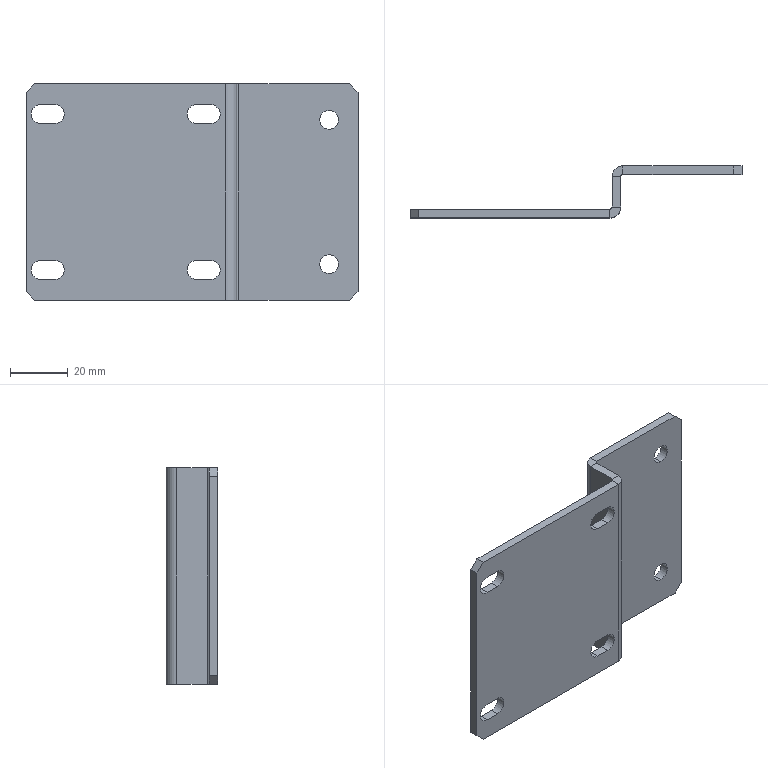Part | STEP file | 1 solid | 46 faces | box 115 x 18 x 75 mm | volume 27777 mm3 | plane 30 | cylinder 16 | commonest cylinder face diameters 6.5 x12 1.473 x2 7.473 x2